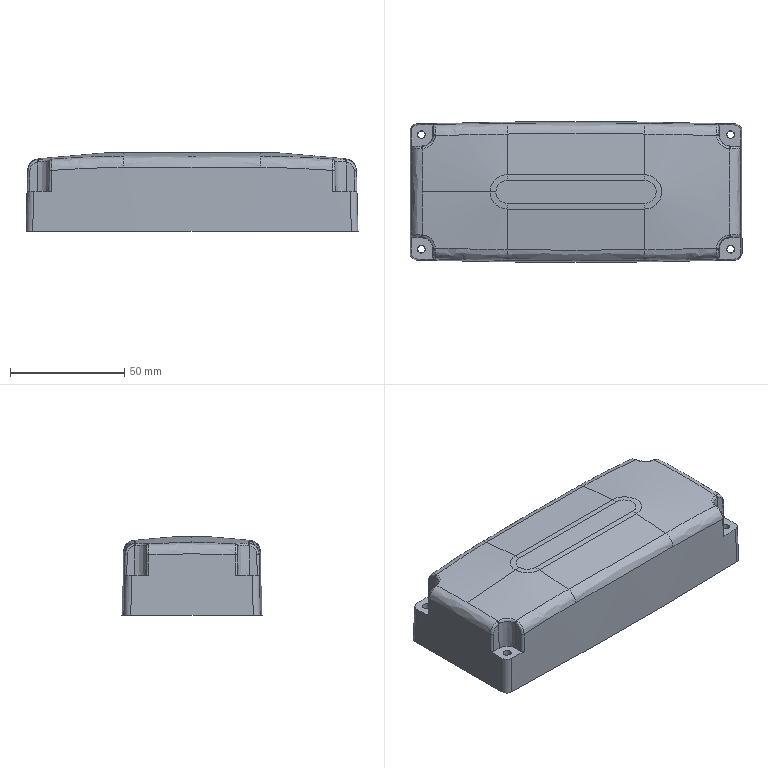Part | SolidWorks | features BaseBody 1 | 1 solid | 80 faces | box 145.001 x 61.5 x 34.5 mm | volume 279097 mm3 | spline 39 | plane 18 | cone 17 | cylinder 6 | commonest cylinder face diameters 2 x4 60 x2